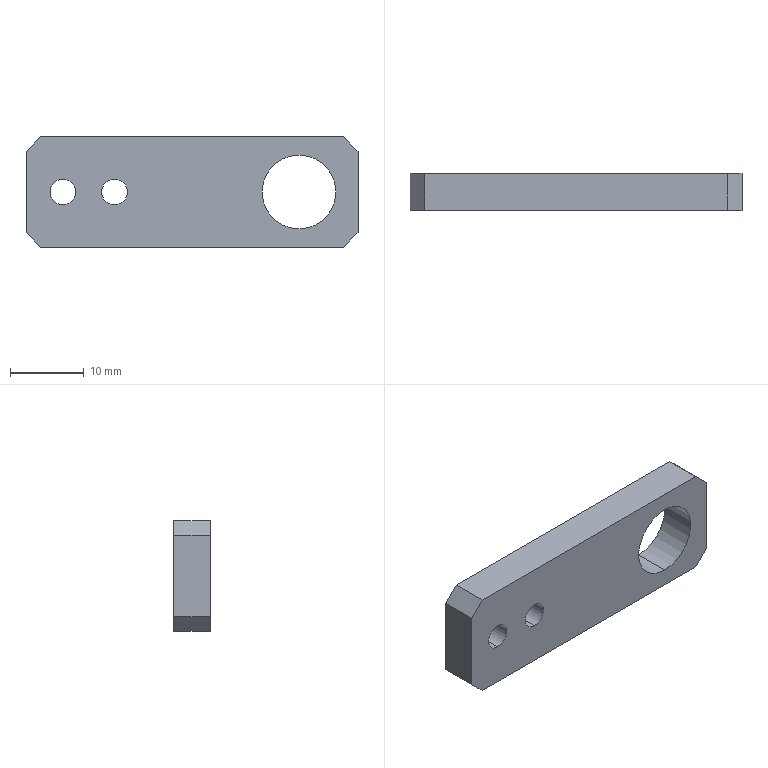Part | STEP file | Extension spring wire fixing bracket 1001 | 1 solid | 16 faces | box 45 x 5 x 15 mm | volume 2846 mm3 | plane 10 | cylinder 6 | commonest cylinder face diameters 3.5 x4 10 x2
STEP:
#1=CARTESIAN_POINT('',(0.,0.,0.));
#2=DIRECTION('',(0.,0.,1.));
#3=DIRECTION('',(1.,0.,0.));
#4=AXIS2_PLACEMENT_3D('',#1,#2,#3);
#5=CARTESIAN_POINT('',(-17.5,0.,1.75));
#6=VERTEX_POINT('',#5);
#7=CARTESIAN_POINT('',(-17.5,5.,1.75));
#8=VERTEX_POINT('',#7);
#9=CARTESIAN_POINT('',(-17.5,0.,1.75));
#10=DIRECTION('',(0.,1.,0.));
#11=VECTOR('',#10,1.);
#12=LINE('',#9,#11);
#13=CARTESIAN_POINT('',(-17.5,0.,0.));
#14=DIRECTION('',(0.,1.,0.));
#15=DIRECTION('',(0.,0.,1.));
#16=AXIS2_PLACEMENT_3D('',#13,#14,#15);
#17=CYLINDRICAL_SURFACE('',#16,1.75);
#18=CARTESIAN_POINT('',(6.283,0.));
#19=DIRECTION('',(0.,1.));
#20=VECTOR('',#19,1.);
#21=LINE('',#18,#20);
#22=(GEOMETRIC_REPRESENTATION_CONTEXT(2)PARAMETRIC_REPRESENTATION_CONTEXT()REPRESENTATION_CONTEXT('',''));
#23=DEFINITIONAL_REPRESENTATION('',(#21),#22);
#24=PCURVE('',#17,#23);
#25=CARTESIAN_POINT('',(-17.5,0.,0.));
#26=DIRECTION('',(0.,1.,0.));
#27=DIRECTION('',(0.,0.,1.));
#28=AXIS2_PLACEMENT_3D('',#25,#26,#27);
#29=CYLINDRICAL_SURFACE('',#28,1.75);
#30=CARTESIAN_POINT('',(0.,0.));
#31=DIRECTION('',(0.,1.));
#32=VECTOR('',#31,1.);
#33=LINE('',#30,#32);
#34=(GEOMETRIC_REPRESENTATION_CONTEXT(2)PARAMETRIC_REPRESENTATION_CONTEXT()REPRESENTATION_CONTEXT('',''));
#35=DEFINITIONAL_REPRESENTATION('',(#33),#34);
#36=PCURVE('',#29,#35);
#37=SURFACE_CURVE('',#12,(#24,#36),.PCURVE_S1.);
#38=EDGE_CURVE('',#6,#8,#37,.T.);
#39=ORIENTED_EDGE('',*,*,#38,.T.);
#40=CARTESIAN_POINT('',(-17.5,5.,-1.75));
#41=VERTEX_POINT('',#40);
#42=CARTESIAN_POINT('',(-17.5,5.,0.));
#43=DIRECTION('',(0.,1.,0.));
#44=DIRECTION('',(0.,0.,1.));
#45=AXIS2_PLACEMENT_3D('',#42,#43,#44);
#46=CIRCLE('',#45,1.75);
#47=CARTESIAN_POINT('',(0.,5.));
#48=DIRECTION('',(1.,0.));
#49=VECTOR('',#48,1.);
#50=LINE('',#47,#49);
#51=(GEOMETRIC_REPRESENTATION_CONTEXT(2)PARAMETRIC_REPRESENTATION_CONTEXT()REPRESENTATION_CONTEXT('',''));
#52=DEFINITIONAL_REPRESENTATION('',(#50),#51);
#53=PCURVE('',#17,#52);
#54=CARTESIAN_POINT('',(0.,5.,0.));
#55=DIRECTION('',(0.,-1.,0.));
#56=DIRECTION('',(0.,0.,-1.));
#57=AXIS2_PLACEMENT_3D('',#54,#55,#56);
#58=PLANE('',#57);
#59=CARTESIAN_POINT('',(-1.75,-17.5));
#60=CARTESIAN_POINT('',(-1.75,-14.469));
#61=CARTESIAN_POINT('',(0.875,-15.984));
#62=CARTESIAN_POINT('',(3.5,-17.5));
#63=CARTESIAN_POINT('',(0.875,-19.016));
#64=CARTESIAN_POINT('',(-1.75,-20.531));
#65=CARTESIAN_POINT('',(-1.75,-17.5));
#66=(BOUNDED_CURVE()B_SPLINE_CURVE(2,(#59,#60,#61,#62,#63,#64,#65),.UNSPECIFIED.,.T.,.F.)B_SPLINE_CURVE_WITH_KNOTS((1,2,2,2,2,1),(-2.094,0.,2.094,4.189,6.283,8.378),.UNSPECIFIED.)CURVE()GEOMETRIC_REPRESENTATION_ITEM()RATIONAL_B_SPLINE_CURVE((1.,0.5,1.,0.5,1.,0.5,1.))REPRESENTATION_ITEM(''));
#67=(GEOMETRIC_REPRESENTATION_CONTEXT(2)PARAMETRIC_REPRESENTATION_CONTEXT()REPRESENTATION_CONTEXT('',''));
#68=DEFINITIONAL_REPRESENTATION('',(#66),#67);
#69=PCURVE('',#58,#68);
#70=SURFACE_CURVE('',#46,(#53,#69),.PCURVE_S1.);
#71=EDGE_CURVE('',#41,#8,#70,.T.);
#72=ORIENTED_EDGE('',*,*,#71,.F.);
#73=CARTESIAN_POINT('',(-17.5,0.,-1.75));
#74=VERTEX_POINT('',#73);
#75=CARTESIAN_POINT('',(-17.5,0.,-1.75));
#76=DIRECTION('',(0.,1.,0.));
#77=VECTOR('',#76,1.);
#78=LINE('',#75,#77);
#79=CARTESIAN_POINT('',(3.142,0.));
#80=DIRECTION('',(0.,1.));
#81=VECTOR('',#80,1.);
#82=LINE('',#79,#81);
#83=(GEOMETRIC_REPRESENTATION_CONTEXT(2)PARAMETRIC_REPRESENTATION_CONTEXT()REPRESENTATION_CONTEXT('',''));
#84=DEFINITIONAL_REPRESENTATION('',(#82),#83);
#85=PCURVE('',#17,#84);
#86=CARTESIAN_POINT('',(3.142,0.));
#87=DIRECTION('',(0.,1.));
#88=VECTOR('',#87,1.);
#89=LINE('',#86,#88);
#90=(GEOMETRIC_REPRESENTATION_CONTEXT(2)PARAMETRIC_REPRESENTATION_CONTEXT()REPRESENTATION_CONTEXT('',''));
#91=DEFINITIONAL_REPRESENTATION('',(#89),#90);
#92=PCURVE('',#29,#91);
#93=SURFACE_CURVE('',#78,(#85,#92),.PCURVE_S1.);
#94=EDGE_CURVE('',#74,#41,#93,.T.);
#95=ORIENTED_EDGE('',*,*,#94,.F.);
#96=CARTESIAN_POINT('',(-17.5,0.,0.));
#97=DIRECTION('',(0.,1.,0.));
#98=DIRECTION('',(0.,0.,1.));
#99=AXIS2_PLACEMENT_3D('',#96,#97,#98);
#100=CIRCLE('',#99,1.75);
#101=CARTESIAN_POINT('',(0.,0.));
#102=DIRECTION('',(1.,0.));
#103=VECTOR('',#102,1.);
#104=LINE('',#101,#103);
#105=(GEOMETRIC_REPRESENTATION_CONTEXT(2)PARAMETRIC_REPRESENTATION_CONTEXT()REPRESENTATION_CONTEXT('',''));
#106=DEFINITIONAL_REPRESENTATION('',(#104),#105);
#107=PCURVE('',#17,#106);
#108=CARTESIAN_POINT('',(0.,0.,0.));
#109=DIRECTION('',(0.,-1.,0.));
#110=DIRECTION('',(0.,0.,-1.));
#111=AXIS2_PLACEMENT_3D('',#108,#109,#110);
#112=PLANE('',#111);
#113=CARTESIAN_POINT('',(-1.75,-17.5));
#114=CARTESIAN_POINT('',(-1.75,-14.469));
#115=CARTESIAN_POINT('',(0.875,-15.984));
#116=CARTESIAN_POINT('',(3.5,-17.5));
#117=CARTESIAN_POINT('',(0.875,-19.016));
#118=CARTESIAN_POINT('',(-1.75,-20.531));
#119=CARTESIAN_POINT('',(-1.75,-17.5));
#120=(BOUNDED_CURVE()B_SPLINE_CURVE(2,(#113,#114,#115,#116,#117,#118,#119),.UNSPECIFIED.,.T.,.F.)B_SPLINE_CURVE_WITH_KNOTS((1,2,2,2,2,1),(-2.094,0.,2.094,4.189,6.283,8.378),.UNSPECIFIED.)CURVE()GEOMETRIC_REPRESENTATION_ITEM()RATIONAL_B_SPLINE_CURVE((1.,0.5,1.,0.5,1.,0.5,1.))REPRESENTATION_ITEM(''));
#121=(GEOMETRIC_REPRESENTATION_CONTEXT(2)PARAMETRIC_REPRESENTATION_CONTEXT()REPRESENTATION_CONTEXT('',''));
#122=DEFINITIONAL_REPRESENTATION('',(#120),#121);
#123=PCURVE('',#112,#122);
#124=SURFACE_CURVE('',#100,(#107,#123),.PCURVE_S1.);
#125=EDGE_CURVE('',#74,#6,#124,.T.);
#126=ORIENTED_EDGE('',*,*,#125,.T.);
#127=EDGE_LOOP('',(#39,#72,#95,#126));
#128=FACE_BOUND('',#127,.F.);
#129=ADVANCED_FACE('',(#128),#17,.F.);
#130=CARTESIAN_POINT('',(-10.5,0.,1.75));
#131=VERTEX_POINT('',#130);
#132=CARTESIAN_POINT('',(-10.5,5.,1.75));
#133=VERTEX_POINT('',#132);
#134=CARTESIAN_POINT('',(-10.5,0.,1.75));
#135=DIRECTION('',(0.,1.,0.));
#136=VECTOR('',#135,1.);
#137=LINE('',#134,#136);
#138=CARTESIAN_POINT('',(-10.5,0.,0.));
#139=DIRECTION('',(0.,1.,0.));
#140=DIRECTION('',(0.,0.,1.));
#141=AXIS2_PLACEMENT_3D('',#138,#139,#140);
#142=CYLINDRICAL_SURFACE('',#141,1.75);
#143=CARTESIAN_POINT('',(6.283,0.));
#144=DIRECTION('',(0.,1.));
#145=VECTOR('',#144,1.);
#146=LINE('',#143,#145);
#147=(GEOMETRIC_REPRESENTATION_CONTEXT(2)PARAMETRIC_REPRESENTATION_CONTEXT()REPRESENTATION_CONTEXT('',''));
#148=DEFINITIONAL_REPRESENTATION('',(#146),#147);
#149=PCURVE('',#142,#148);
#150=CARTESIAN_POINT('',(-10.5,0.,0.));
#151=DIRECTION('',(0.,1.,0.));
#152=DIRECTION('',(0.,0.,1.));
#153=AXIS2_PLACEMENT_3D('',#150,#151,#152);
#154=CYLINDRICAL_SURFACE('',#153,1.75);
#155=CARTESIAN_POINT('',(0.,0.));
#156=DIRECTION('',(0.,1.));
#157=VECTOR('',#156,1.);
#158=LINE('',#155,#157);
#159=(GEOMETRIC_REPRESENTATION_CONTEXT(2)PARAMETRIC_REPRESENTATION_CONTEXT()REPRESENTATION_CONTEXT('',''));
#160=DEFINITIONAL_REPRESENTATION('',(#158),#159);
#161=PCURVE('',#154,#160);
#162=SURFACE_CURVE('',#137,(#149,#161),.PCURVE_S1.);
#163=EDGE_CURVE('',#131,#133,#162,.T.);
#164=ORIENTED_EDGE('',*,*,#163,.T.);
#165=CARTESIAN_POINT('',(-10.5,5.,-1.75));
#166=VERTEX_POINT('',#165);
#167=CARTESIAN_POINT('',(-10.5,5.,0.));
#168=DIRECTION('',(0.,1.,0.));
#169=DIRECTION('',(0.,0.,1.));
#170=AXIS2_PLACEMENT_3D('',#167,#168,#169);
#171=CIRCLE('',#170,1.75);
#172=CARTESIAN_POINT('',(0.,5.));
#173=DIRECTION('',(1.,0.));
#174=VECTOR('',#173,1.);
#175=LINE('',#172,#174);
#176=(GEOMETRIC_REPRESENTATION_CONTEXT(2)PARAMETRIC_REPRESENTATION_CONTEXT()REPRESENTATION_CONTEXT('',''));
#177=DEFINITIONAL_REPRESENTATION('',(#175),#176);
#178=PCURVE('',#142,#177);
#179=CARTESIAN_POINT('',(-1.75,-10.5));
#180=CARTESIAN_POINT('',(-1.75,-7.469));
#181=CARTESIAN_POINT('',(0.875,-8.984));
#182=CARTESIAN_POINT('',(3.5,-10.5));
#183=CARTESIAN_POINT('',(0.875,-12.016));
#184=CARTESIAN_POINT('',(-1.75,-13.531));
#185=CARTESIAN_POINT('',(-1.75,-10.5));
#186=(BOUNDED_CURVE()B_SPLINE_CURVE(2,(#179,#180,#181,#182,#183,#184,#185),.UNSPECIFIED.,.T.,.F.)B_SPLINE_CURVE_WITH_KNOTS((1,2,2,2,2,1),(-2.094,0.,2.094,4.189,6.283,8.378),.UNSPECIFIED.)CURVE()GEOMETRIC_REPRESENTATION_ITEM()RATIONAL_B_SPLINE_CURVE((1.,0.5,1.,0.5,1.,0.5,1.))REPRESENTATION_ITEM(''));
#187=(GEOMETRIC_REPRESENTATION_CONTEXT(2)PARAMETRIC_REPRESENTATION_CONTEXT()REPRESENTATION_CONTEXT('',''));
#188=DEFINITIONAL_REPRESENTATION('',(#186),#187);
#189=PCURVE('',#58,#188);
#190=SURFACE_CURVE('',#171,(#178,#189),.PCURVE_S1.);
#191=EDGE_CURVE('',#166,#133,#190,.T.);
#192=ORIENTED_EDGE('',*,*,#191,.F.);
#193=CARTESIAN_POINT('',(-10.5,0.,-1.75));
#194=VERTEX_POINT('',#193);
#195=CARTESIAN_POINT('',(-10.5,0.,-1.75));
#196=DIRECTION('',(0.,1.,0.));
#197=VECTOR('',#196,1.);
#198=LINE('',#195,#197);
#199=CARTESIAN_POINT('',(3.142,0.));
#200=DIRECTION('',(0.,1.));
#201=VECTOR('',#200,1.);
#202=LINE('',#199,#201);
#203=(GEOMETRIC_REPRESENTATION_CONTEXT(2)PARAMETRIC_REPRESENTATION_CONTEXT()REPRESENTATION_CONTEXT('',''));
#204=DEFINITIONAL_REPRESENTATION('',(#202),#203);
#205=PCURVE('',#142,#204);
#206=CARTESIAN_POINT('',(3.142,0.));
#207=DIRECTION('',(0.,1.));
#208=VECTOR('',#207,1.);
#209=LINE('',#206,#208);
#210=(GEOMETRIC_REPRESENTATION_CONTEXT(2)PARAMETRIC_REPRESENTATION_CONTEXT()REPRESENTATION_CONTEXT('',''));
#211=DEFINITIONAL_REPRESENTATION('',(#209),#210);
#212=PCURVE('',#154,#211);
#213=SURFACE_CURVE('',#198,(#205,#212),.PCURVE_S1.);
#214=EDGE_CURVE('',#194,#166,#213,.T.);
#215=ORIENTED_EDGE('',*,*,#214,.F.);
#216=CARTESIAN_POINT('',(-10.5,0.,0.));
#217=DIRECTION('',(0.,1.,0.));
#218=DIRECTION('',(0.,0.,1.));
#219=AXIS2_PLACEMENT_3D('',#216,#217,#218);
#220=CIRCLE('',#219,1.75);
#221=CARTESIAN_POINT('',(0.,0.));
#222=DIRECTION('',(1.,0.));
#223=VECTOR('',#222,1.);
#224=LINE('',#221,#223);
#225=(GEOMETRIC_REPRESENTATION_CONTEXT(2)PARAMETRIC_REPRESENTATION_CONTEXT()REPRESENTATION_CONTEXT('',''));
#226=DEFINITIONAL_REPRESENTATION('',(#224),#225);
#227=PCURVE('',#142,#226);
#228=CARTESIAN_POINT('',(-1.75,-10.5));
#229=CARTESIAN_POINT('',(-1.75,-7.469));
#230=CARTESIAN_POINT('',(0.875,-8.984));
#231=CARTESIAN_POINT('',(3.5,-10.5));
#232=CARTESIAN_POINT('',(0.875,-12.016));
#233=CARTESIAN_POINT('',(-1.75,-13.531));
#234=CARTESIAN_POINT('',(-1.75,-10.5));
#235=(BOUNDED_CURVE()B_SPLINE_CURVE(2,(#228,#229,#230,#231,#232,#233,#234),.UNSPECIFIED.,.T.,.F.)B_SPLINE_CURVE_WITH_KNOTS((1,2,2,2,2,1),(-2.094,0.,2.094,4.189,6.283,8.378),.UNSPECIFIED.)CURVE()GEOMETRIC_REPRESENTATION_ITEM()RATIONAL_B_SPLINE_CURVE((1.,0.5,1.,0.5,1.,0.5,1.))REPRESENTATION_ITEM(''));
#236=(GEOMETRIC_REPRESENTATION_CONTEXT(2)PARAMETRIC_REPRESENTATION_CONTEXT()REPRESENTATION_CONTEXT('',''));
#237=DEFINITIONAL_REPRESENTATION('',(#235),#236);
#238=PCURVE('',#112,#237);
#239=SURFACE_CURVE('',#220,(#227,#238),.PCURVE_S1.);
#240=EDGE_CURVE('',#194,#131,#239,.T.);
#241=ORIENTED_EDGE('',*,*,#240,.T.);
#242=EDGE_LOOP('',(#164,#192,#215,#241));
#243=FACE_BOUND('',#242,.F.);
#244=ADVANCED_FACE('',(#243),#142,.F.);
#245=CARTESIAN_POINT('',(14.5,0.,5.));
#246=VERTEX_POINT('',#245);
#247=CARTESIAN_POINT('',(14.5,5.,5.));
#248=VERTEX_POINT('',#247);
#249=CARTESIAN_POINT('',(14.5,0.,5.));
#250=DIRECTION('',(0.,1.,0.));
#251=VECTOR('',#250,1.);
#252=LINE('',#249,#251);
#253=CARTESIAN_POINT('',(14.5,0.,0.));
#254=DIRECTION('',(0.,1.,0.));
#255=DIRECTION('',(0.,0.,1.));
#256=AXIS2_PLACEMENT_3D('',#253,#254,#255);
#257=CYLINDRICAL_SURFACE('',#256,5.);
#258=CARTESIAN_POINT('',(6.283,0.));
#259=DIRECTION('',(0.,1.));
#260=VECTOR('',#259,1.);
#261=LINE('',#258,#260);
#262=(GEOMETRIC_REPRESENTATION_CONTEXT(2)PARAMETRIC_REPRESENTATION_CONTEXT()REPRESENTATION_CONTEXT('',''));
#263=DEFINITIONAL_REPRESENTATION('',(#261),#262);
#264=PCURVE('',#257,#263);
#265=CARTESIAN_POINT('',(14.5,0.,0.));
#266=DIRECTION('',(0.,1.,0.));
#267=DIRECTION('',(0.,0.,1.));
#268=AXIS2_PLACEMENT_3D('',#265,#266,#267);
#269=CYLINDRICAL_SURFACE('',#268,5.);
#270=CARTESIAN_POINT('',(0.,0.));
#271=DIRECTION('',(0.,1.));
#272=VECTOR('',#271,1.);
#273=LINE('',#270,#272);
#274=(GEOMETRIC_REPRESENTATION_CONTEXT(2)PARAMETRIC_REPRESENTATION_CONTEXT()REPRESENTATION_CONTEXT('',''));
#275=DEFINITIONAL_REPRESENTATION('',(#273),#274);
#276=PCURVE('',#269,#275);
#277=SURFACE_CURVE('',#252,(#264,#276),.PCURVE_S1.);
#278=EDGE_CURVE('',#246,#248,#277,.T.);
#279=ORIENTED_EDGE('',*,*,#278,.T.);
#280=CARTESIAN_POINT('',(14.5,5.,-5.));
#281=VERTEX_POINT('',#280);
#282=CARTESIAN_POINT('',(14.5,5.,0.));
#283=DIRECTION('',(0.,1.,0.));
#284=DIRECTION('',(0.,0.,1.));
#285=AXIS2_PLACEMENT_3D('',#282,#283,#284);
#286=CIRCLE('',#285,5.);
#287=CARTESIAN_POINT('',(0.,5.));
#288=DIRECTION('',(1.,0.));
#289=VECTOR('',#288,1.);
#290=LINE('',#287,#289);
#291=(GEOMETRIC_REPRESENTATION_CONTEXT(2)PARAMETRIC_REPRESENTATION_CONTEXT()REPRESENTATION_CONTEXT('',''));
#292=DEFINITIONAL_REPRESENTATION('',(#290),#291);
#293=PCURVE('',#257,#292);
#294=CARTESIAN_POINT('',(-5.,14.5));
#295=CARTESIAN_POINT('',(-5.,23.16));
#296=CARTESIAN_POINT('',(2.5,18.83));
#297=CARTESIAN_POINT('',(10.,14.5));
#298=CARTESIAN_POINT('',(2.5,10.17));
#299=CARTESIAN_POINT('',(-5.,5.84));
#300=CARTESIAN_POINT('',(-5.,14.5));
#301=(BOUNDED_CURVE()B_SPLINE_CURVE(2,(#294,#295,#296,#297,#298,#299,#300),.UNSPECIFIED.,.T.,.F.)B_SPLINE_CURVE_WITH_KNOTS((1,2,2,2,2,1),(-2.094,0.,2.094,4.189,6.283,8.378),.UNSPECIFIED.)CURVE()GEOMETRIC_REPRESENTATION_ITEM()RATIONAL_B_SPLINE_CURVE((1.,0.5,1.,0.5,1.,0.5,1.))REPRESENTATION_ITEM(''));
#302=(GEOMETRIC_REPRESENTATION_CONTEXT(2)PARAMETRIC_REPRESENTATION_CONTEXT()REPRESENTATION_CONTEXT('',''));
#303=DEFINITIONAL_REPRESENTATION('',(#301),#302);
#304=PCURVE('',#58,#303);
#305=SURFACE_CURVE('',#286,(#293,#304),.PCURVE_S1.);
#306=EDGE_CURVE('',#281,#248,#305,.T.);
#307=ORIENTED_EDGE('',*,*,#306,.F.);
#308=CARTESIAN_POINT('',(14.5,0.,-5.));
#309=VERTEX_POINT('',#308);
#310=CARTESIAN_POINT('',(14.5,0.,-5.));
#311=DIRECTION('',(0.,1.,0.));
#312=VECTOR('',#311,1.);
#313=LINE('',#310,#312);
#314=CARTESIAN_POINT('',(3.142,0.));
#315=DIRECTION('',(0.,1.));
#316=VECTOR('',#315,1.);
#317=LINE('',#314,#316);
#318=(GEOMETRIC_REPRESENTATION_CONTEXT(2)PARAMETRIC_REPRESENTATION_CONTEXT()REPRESENTATION_CONTEXT('',''));
#319=DEFINITIONAL_REPRESENTATION('',(#317),#318);
#320=PCURVE('',#257,#319);
#321=CARTESIAN_POINT('',(3.142,0.));
#322=DIRECTION('',(0.,1.));
#323=VECTOR('',#322,1.);
#324=LINE('',#321,#323);
#325=(GEOMETRIC_REPRESENTATION_CONTEXT(2)PARAMETRIC_REPRESENTATION_CONTEXT()REPRESENTATION_CONTEXT('',''));
#326=DEFINITIONAL_REPRESENTATION('',(#324),#325);
#327=PCURVE('',#269,#326);
#328=SURFACE_CURVE('',#313,(#320,#327),.PCURVE_S1.);
#329=EDGE_CURVE('',#309,#281,#328,.T.);
#330=ORIENTED_EDGE('',*,*,#329,.F.);
#331=CARTESIAN_POINT('',(14.5,0.,0.));
#332=DIRECTION('',(0.,1.,0.));
#333=DIRECTION('',(0.,0.,1.));
#334=AXIS2_PLACEMENT_3D('',#331,#332,#333);
#335=CIRCLE('',#334,5.);
#336=CARTESIAN_POINT('',(0.,0.));
#337=DIRECTION('',(1.,0.));
#338=VECTOR('',#337,1.);
#339=LINE('',#336,#338);
#340=(GEOMETRIC_REPRESENTATION_CONTEXT(2)PARAMETRIC_REPRESENTATION_CONTEXT()REPRESENTATION_CONTEXT('',''));
#341=DEFINITIONAL_REPRESENTATION('',(#339),#340);
#342=PCURVE('',#257,#341);
#343=CARTESIAN_POINT('',(-5.,14.5));
#344=CARTESIAN_POINT('',(-5.,23.16));
#345=CARTESIAN_POINT('',(2.5,18.83));
#346=CARTESIAN_POINT('',(10.,14.5));
#347=CARTESIAN_POINT('',(2.5,10.17));
#348=CARTESIAN_POINT('',(-5.,5.84));
#349=CARTESIAN_POINT('',(-5.,14.5));
#350=(BOUNDED_CURVE()B_SPLINE_CURVE(2,(#343,#344,#345,#346,#347,#348,#349),.UNSPECIFIED.,.T.,.F.)B_SPLINE_CURVE_WITH_KNOTS((1,2,2,2,2,1),(-2.094,0.,2.094,4.189,6.283,8.378),.UNSPECIFIED.)CURVE()GEOMETRIC_REPRESENTATION_ITEM()RATIONAL_B_SPLINE_CURVE((1.,0.5,1.,0.5,1.,0.5,1.))REPRESENTATION_ITEM(''));
#351=(GEOMETRIC_REPRESENTATION_CONTEXT(2)PARAMETRIC_REPRESENTATION_CONTEXT()REPRESENTATION_CONTEXT('',''));
#352=DEFINITIONAL_REPRESENTATION('',(#350),#351);
#353=PCURVE('',#112,#352);
#354=SURFACE_CURVE('',#335,(#342,#353),.PCURVE_S1.);
#355=EDGE_CURVE('',#309,#246,#354,.T.);
#356=ORIENTED_EDGE('',*,*,#355,.T.);
#357=EDGE_LOOP('',(#279,#307,#330,#356));
#358=FACE_BOUND('',#357,.F.);
#359=ADVANCED_FACE('',(#358),#257,.F.);
#360=CARTESIAN_POINT('',(22.5,5.,5.5));
#361=VERTEX_POINT('',#360);
#362=CARTESIAN_POINT('',(22.5,5.,-5.5));
#363=VERTEX_POINT('',#362);
#364=CARTESIAN_POINT('',(22.5,5.,7.5));
#365=DIRECTION('',(0.,0.,-1.));
#366=VECTOR('',#365,1.);
#367=LINE('',#364,#366);
#368=CARTESIAN_POINT('',(22.5,5.,7.5));
#369=DIRECTION('',(-1.,0.,0.));
#370=DIRECTION('',(0.,0.,1.));
#371=AXIS2_PLACEMENT_3D('',#368,#369,#370);
#372=PLANE('',#371);
#373=CARTESIAN_POINT('',(0.,0.));
#374=DIRECTION('',(-1.,0.));
#375=VECTOR('',#374,1.);
#376=LINE('',#373,#375);
#377=(GEOMETRIC_REPRESENTATION_CONTEXT(2)PARAMETRIC_REPRESENTATION_CONTEXT()REPRESENTATION_CONTEXT('',''));
#378=DEFINITIONAL_REPRESENTATION('',(#376),#377);
#379=PCURVE('',#372,#378);
#380=CARTESIAN_POINT('',(-7.5,22.5));
#381=DIRECTION('',(1.,0.));
#382=VECTOR('',#381,1.);
#383=LINE('',#380,#382);
#384=(GEOMETRIC_REPRESENTATION_CONTEXT(2)PARAMETRIC_REPRESENTATION_CONTEXT()REPRESENTATION_CONTEXT('',''));
#385=DEFINITIONAL_REPRESENTATION('',(#383),#384);
#386=PCURVE('',#58,#385);
#387=SURFACE_CURVE('',#367,(#379,#386),.PCURVE_S1.);
#388=EDGE_CURVE('',#361,#363,#387,.T.);
#389=ORIENTED_EDGE('',*,*,#388,.F.);
#390=CARTESIAN_POINT('',(22.5,0.,5.5));
#391=VERTEX_POINT('',#390);
#392=CARTESIAN_POINT('',(22.5,5.,5.5));
#393=DIRECTION('',(0.,-1.,0.));
#394=VECTOR('',#393,1.);
#395=LINE('',#392,#394);
#396=CARTESIAN_POINT('',(-2.,0.));
#397=DIRECTION('',(0.,-1.));
#398=VECTOR('',#397,1.);
#399=LINE('',#396,#398);
#400=(GEOMETRIC_REPRESENTATION_CONTEXT(2)PARAMETRIC_REPRESENTATION_CONTEXT()REPRESENTATION_CONTEXT('',''));
#401=DEFINITIONAL_REPRESENTATION('',(#399),#400);
#402=PCURVE('',#372,#401);
#403=CARTESIAN_POINT('',(22.5,5.,5.5));
#404=DIRECTION('',(-0.7071,0.,-0.7071));
#405=DIRECTION('',(0.,-1.,0.));
#406=AXIS2_PLACEMENT_3D('',#403,#404,#405);
#407=PLANE('',#406);
#408=CARTESIAN_POINT('',(0.,0.));
#409=DIRECTION('',(1.,0.));
#410=VECTOR('',#409,1.);
#411=LINE('',#408,#410);
#412=(GEOMETRIC_REPRESENTATION_CONTEXT(2)PARAMETRIC_REPRESENTATION_CONTEXT()REPRESENTATION_CONTEXT('',''));
#413=DEFINITIONAL_REPRESENTATION('',(#411),#412);
#414=PCURVE('',#407,#413);
#415=SURFACE_CURVE('',#395,(#402,#414),.PCURVE_S1.);
#416=EDGE_CURVE('',#361,#391,#415,.T.);
#417=ORIENTED_EDGE('',*,*,#416,.T.);
#418=CARTESIAN_POINT('',(22.5,0.,-5.5));
#419=VERTEX_POINT('',#418);
#420=CARTESIAN_POINT('',(22.5,0.,7.5));
#421=DIRECTION('',(0.,0.,-1.));
#422=VECTOR('',#421,1.);
#423=LINE('',#420,#422);
#424=CARTESIAN_POINT('',(0.,-5.));
#425=DIRECTION('',(-1.,0.));
#426=VECTOR('',#425,1.);
#427=LINE('',#424,#426);
#428=(GEOMETRIC_REPRESENTATION_CONTEXT(2)PARAMETRIC_REPRESENTATION_CONTEXT()REPRESENTATION_CONTEXT('',''));
#429=DEFINITIONAL_REPRESENTATION('',(#427),#428);
#430=PCURVE('',#372,#429);
#431=CARTESIAN_POINT('',(-7.5,22.5));
#432=DIRECTION('',(1.,0.));
#433=VECTOR('',#432,1.);
#434=LINE('',#431,#433);
#435=(GEOMETRIC_REPRESENTATION_CONTEXT(2)PARAMETRIC_REPRESENTATION_CONTEXT()REPRESENTATION_CONTEXT('',''));
#436=DEFINITIONAL_REPRESENTATION('',(#434),#435);
#437=PCURVE('',#112,#436);
#438=SURFACE_CURVE('',#423,(#430,#437),.PCURVE_S1.);
#439=EDGE_CURVE('',#391,#419,#438,.T.);
#440=ORIENTED_EDGE('',*,*,#439,.T.);
#441=CARTESIAN_POINT('',(22.5,5.,-5.5));
#442=DIRECTION('',(0.,1.,0.));
#443=VECTOR('',#442,1.);
#444=LINE('',#441,#443);
#445=CARTESIAN_POINT('',(-13.,0.));
#446=DIRECTION('',(0.,1.));
#447=VECTOR('',#446,1.);
#448=LINE('',#445,#447);
#449=(GEOMETRIC_REPRESENTATION_CONTEXT(2)PARAMETRIC_REPRESENTATION_CONTEXT()REPRESENTATION_CONTEXT('',''));
#450=DEFINITIONAL_REPRESENTATION('',(#448),#449);
#451=PCURVE('',#372,#450);
#452=CARTESIAN_POINT('',(20.5,5.,-7.5));
#453=DIRECTION('',(-0.7071,0.,0.7071));
#454=DIRECTION('',(0.,-1.,0.));
#455=AXIS2_PLACEMENT_3D('',#452,#453,#454);
#456=PLANE('',#455);
#457=CARTESIAN_POINT('',(0.,2.828));
#458=DIRECTION('',(-1.,0.));
#459=VECTOR('',#458,1.);
#460=LINE('',#457,#459);
#461=(GEOMETRIC_REPRESENTATION_CONTEXT(2)PARAMETRIC_REPRESENTATION_CONTEXT()REPRESENTATION_CONTEXT('',''));
#462=DEFINITIONAL_REPRESENTATION('',(#460),#461);
#463=PCURVE('',#456,#462);
#464=SURFACE_CURVE('',#444,(#451,#463),.PCURVE_S1.);
#465=EDGE_CURVE('',#419,#363,#464,.T.);
#466=ORIENTED_EDGE('',*,*,#465,.T.);
#467=EDGE_LOOP('',(#389,#417,#440,#466));
#468=FACE_BOUND('',#467,.T.);
#469=ADVANCED_FACE('',(#468),#372,.F.);
#470=CARTESIAN_POINT('',(20.5,0.,-7.5));
#471=VERTEX_POINT('',#470);
#472=CARTESIAN_POINT('',(-20.5,0.,-7.5));
#473=VERTEX_POINT('',#472);
#474=CARTESIAN_POINT('',(-22.5,0.,-7.5));
#475=DIRECTION('',(-1.,0.,0.));
#476=VECTOR('',#475,1.);
#477=LINE('',#474,#476);
#478=CARTESIAN_POINT('',(-22.5,5.,-7.5));
#479=DIRECTION('',(0.,0.,1.));
#480=DIRECTION('',(1.,0.,0.));
#481=AXIS2_PLACEMENT_3D('',#478,#479,#480);
#482=PLANE('',#481);
#483=CARTESIAN_POINT('',(0.,-5.));
#484=DIRECTION('',(-1.,0.));
#485=VECTOR('',#484,1.);
#486=LINE('',#483,#485);
#487=(GEOMETRIC_REPRESENTATION_CONTEXT(2)PARAMETRIC_REPRESENTATION_CONTEXT()REPRESENTATION_CONTEXT('',''));
#488=DEFINITIONAL_REPRESENTATION('',(#486),#487);
#489=PCURVE('',#482,#488);
#490=CARTESIAN_POINT('',(7.5,-22.5));
#491=DIRECTION('',(0.,-1.));
#492=VECTOR('',#491,1.);
#493=LINE('',#490,#492);
#494=(GEOMETRIC_REPRESENTATION_CONTEXT(2)PARAMETRIC_REPRESENTATION_CONTEXT()REPRESENTATION_CONTEXT('',''));
#495=DEFINITIONAL_REPRESENTATION('',(#493),#494);
#496=PCURVE('',#112,#495);
#497=SURFACE_CURVE('',#477,(#489,#496),.PCURVE_S1.);
#498=EDGE_CURVE('',#471,#473,#497,.T.);
#499=ORIENTED_EDGE('',*,*,#498,.T.);
#500=CARTESIAN_POINT('',(-20.5,5.,-7.5));
#501=VERTEX_POINT('',#500);
#502=CARTESIAN_POINT('',(-20.5,5.,-7.5));
#503=DIRECTION('',(0.,1.,0.));
#504=VECTOR('',#503,1.);
#505=LINE('',#502,#504);
#506=CARTESIAN_POINT('',(2.,0.));
#507=DIRECTION('',(0.,1.));
#508=VECTOR('',#507,1.);
#509=LINE('',#506,#508);
#510=(GEOMETRIC_REPRESENTATION_CONTEXT(2)PARAMETRIC_REPRESENTATION_CONTEXT()REPRESENTATION_CONTEXT('',''));
#511=DEFINITIONAL_REPRESENTATION('',(#509),#510);
#512=PCURVE('',#482,#511);
#513=CARTESIAN_POINT('',(-22.5,5.,-5.5));
#514=DIRECTION('',(0.7071,0.,0.7071));
#515=DIRECTION('',(0.,-1.,0.));
#516=AXIS2_PLACEMENT_3D('',#513,#514,#515);
#517=PLANE('',#516);
#518=CARTESIAN_POINT('',(0.,2.828));
#519=DIRECTION('',(-1.,0.));
#520=VECTOR('',#519,1.);
#521=LINE('',#518,#520);
#522=(GEOMETRIC_REPRESENTATION_CONTEXT(2)PARAMETRIC_REPRESENTATION_CONTEXT()REPRESENTATION_CONTEXT('',''));
#523=DEFINITIONAL_REPRESENTATION('',(#521),#522);
#524=PCURVE('',#517,#523);
#525=SURFACE_CURVE('',#505,(#512,#524),.PCURVE_S1.);
#526=EDGE_CURVE('',#473,#501,#525,.T.);
#527=ORIENTED_EDGE('',*,*,#526,.T.);
#528=CARTESIAN_POINT('',(20.5,5.,-7.5));
#529=VERTEX_POINT('',#528);
#530=CARTESIAN_POINT('',(-22.5,5.,-7.5));
#531=DIRECTION('',(-1.,0.,0.));
#532=VECTOR('',#531,1.);
#533=LINE('',#530,#532);
#534=CARTESIAN_POINT('',(0.,0.));
#535=DIRECTION('',(-1.,0.));
#536=VECTOR('',#535,1.);
#537=LINE('',#534,#536);
#538=(GEOMETRIC_REPRESENTATION_CONTEXT(2)PARAMETRIC_REPRESENTATION_CONTEXT()REPRESENTATION_CONTEXT('',''));
#539=DEFINITIONAL_REPRESENTATION('',(#537),#538);
#540=PCURVE('',#482,#539);
#541=CARTESIAN_POINT('',(7.5,-22.5));
#542=DIRECTION('',(0.,-1.));
#543=VECTOR('',#542,1.);
#544=LINE('',#541,#543);
#545=(GEOMETRIC_REPRESENTATION_CONTEXT(2)PARAMETRIC_REPRESENTATION_CONTEXT()REPRESENTATION_CONTEXT('',''));
#546=DEFINITIONAL_REPRESENTATION('',(#544),#545);
#547=PCURVE('',#58,#546);
#548=SURFACE_CURVE('',#533,(#540,#547),.PCURVE_S1.);
#549=EDGE_CURVE('',#529,#501,#548,.T.);
#550=ORIENTED_EDGE('',*,*,#549,.F.);
#551=CARTESIAN_POINT('',(20.5,5.,-7.5));
#552=DIRECTION('',(0.,-1.,0.));
#553=VECTOR('',#552,1.);
#554=LINE('',#551,#553);
#555=CARTESIAN_POINT('',(43.,0.));
#556=DIRECTION('',(0.,-1.));
#557=VECTOR('',#556,1.);
#558=LINE('',#555,#557);
#559=(GEOMETRIC_REPRESENTATION_CONTEXT(2)PARAMETRIC_REPRESENTATION_CONTEXT()REPRESENTATION_CONTEXT('',''));
#560=DEFINITIONAL_REPRESENTATION('',(#558),#559);
#561=PCURVE('',#482,#560);
#562=CARTESIAN_POINT('',(0.,0.));
#563=DIRECTION('',(1.,0.));
#564=VECTOR('',#563,1.);
#565=LINE('',#562,#564);
#566=(GEOMETRIC_REPRESENTATION_CONTEXT(2)PARAMETRIC_REPRESENTATION_CONTEXT()REPRESENTATION_CONTEXT('',''));
#567=DEFINITIONAL_REPRESENTATION('',(#565),#566);
#568=PCURVE('',#456,#567);
#569=SURFACE_CURVE('',#554,(#561,#568),.PCURVE_S1.);
#570=EDGE_CURVE('',#529,#471,#569,.T.);
#571=ORIENTED_EDGE('',*,*,#570,.T.);
#572=EDGE_LOOP('',(#499,#527,#550,#571));
#573=FACE_BOUND('',#572,.T.);
#574=ADVANCED_FACE('',(#573),#482,.F.);
#575=CARTESIAN_POINT('',(-22.5,0.,-5.5));
#576=VERTEX_POINT('',#575);
#577=CARTESIAN_POINT('',(-22.5,0.,5.5));
#578=VERTEX_POINT('',#577);
#579=CARTESIAN_POINT('',(-22.5,0.,7.5));
#580=DIRECTION('',(0.,0.,1.));
#581=VECTOR('',#580,1.);
#582=LINE('',#579,#581);
#583=CARTESIAN_POINT('',(-22.5,5.,7.5));
#584=DIRECTION('',(1.,0.,0.));
#585=DIRECTION('',(0.,0.,-1.));
#586=AXIS2_PLACEMENT_3D('',#583,#584,#585);
#587=PLANE('',#586);
#588=CARTESIAN_POINT('',(0.,-5.));
#589=DIRECTION('',(-1.,0.));
#590=VECTOR('',#589,1.);
#591=LINE('',#588,#590);
#592=(GEOMETRIC_REPRESENTATION_CONTEXT(2)PARAMETRIC_REPRESENTATION_CONTEXT()REPRESENTATION_CONTEXT('',''));
#593=DEFINITIONAL_REPRESENTATION('',(#591),#592);
#594=PCURVE('',#587,#593);
#595=CARTESIAN_POINT('',(-7.5,-22.5));
#596=DIRECTION('',(-1.,0.));
#597=VECTOR('',#596,1.);
#598=LINE('',#595,#597);
#599=(GEOMETRIC_REPRESENTATION_CONTEXT(2)PARAMETRIC_REPRESENTATION_CONTEXT()REPRESENTATION_CONTEXT('',''));
#600=DEFINITIONAL_REPRESENTATION('',(#598),#599);
#601=PCURVE('',#112,#600);
#602=SURFACE_CURVE('',#582,(#594,#601),.PCURVE_S1.);
#603=EDGE_CURVE('',#576,#578,#602,.T.);
#604=ORIENTED_EDGE('',*,*,#603,.T.);
#605=CARTESIAN_POINT('',(-22.5,5.,5.5));
#606=VERTEX_POINT('',#605);
#607=CARTESIAN_POINT('',(-22.5,5.,5.5));
#608=DIRECTION('',(0.,1.,0.));
#609=VECTOR('',#608,1.);
#610=LINE('',#607,#609);
#611=CARTESIAN_POINT('',(2.,0.));
#612=DIRECTION('',(0.,1.));
#613=VECTOR('',#612,1.);
#614=LINE('',#611,#613);
#615=(GEOMETRIC_REPRESENTATION_CONTEXT(2)PARAMETRIC_REPRESENTATION_CONTEXT()REPRESENTATION_CONTEXT('',''));
#616=DEFINITIONAL_REPRESENTATION('',(#614),#615);
#617=PCURVE('',#587,#616);
#618=CARTESIAN_POINT('',(-20.5,5.,7.5));
#619=DIRECTION('',(0.7071,0.,-0.7071));
#620=DIRECTION('',(0.,-1.,0.));
#621=AXIS2_PLACEMENT_3D('',#618,#619,#620);
#622=PLANE('',#621);
#623=CARTESIAN_POINT('',(0.,2.828));
#624=DIRECTION('',(-1.,0.));
#625=VECTOR('',#624,1.);
#626=LINE('',#623,#625);
#627=(GEOMETRIC_REPRESENTATION_CONTEXT(2)PARAMETRIC_REPRESENTATION_CONTEXT()REPRESENTATION_CONTEXT('',''));
#628=DEFINITIONAL_REPRESENTATION('',(#626),#627);
#629=PCURVE('',#622,#628);
#630=SURFACE_CURVE('',#610,(#617,#629),.PCURVE_S1.);
#631=EDGE_CURVE('',#578,#606,#630,.T.);
#632=ORIENTED_EDGE('',*,*,#631,.T.);
#633=CARTESIAN_POINT('',(-22.5,5.,-5.5));
#634=VERTEX_POINT('',#633);
#635=CARTESIAN_POINT('',(-22.5,5.,7.5));
#636=DIRECTION('',(0.,0.,1.));
#637=VECTOR('',#636,1.);
#638=LINE('',#635,#637);
#639=CARTESIAN_POINT('',(0.,0.));
#640=DIRECTION('',(-1.,0.));
#641=VECTOR('',#640,1.);
#642=LINE('',#639,#641);
#643=(GEOMETRIC_REPRESENTATION_CONTEXT(2)PARAMETRIC_REPRESENTATION_CONTEXT()REPRESENTATION_CONTEXT('',''));
#644=DEFINITIONAL_REPRESENTATION('',(#642),#643);
#645=PCURVE('',#587,#644);
#646=CARTESIAN_POINT('',(-7.5,-22.5));
#647=DIRECTION('',(-1.,0.));
#648=VECTOR('',#647,1.);
#649=LINE('',#646,#648);
#650=(GEOMETRIC_REPRESENTATION_CONTEXT(2)PARAMETRIC_REPRESENTATION_CONTEXT()REPRESENTATION_CONTEXT('',''));
#651=DEFINITIONAL_REPRESENTATION('',(#649),#650);
#652=PCURVE('',#58,#651);
#653=SURFACE_CURVE('',#638,(#645,#652),.PCURVE_S1.);
#654=EDGE_CURVE('',#634,#606,#653,.T.);
#655=ORIENTED_EDGE('',*,*,#654,.F.);
#656=CARTESIAN_POINT('',(-22.5,5.,-5.5));
#657=DIRECTION('',(0.,-1.,0.));
#658=VECTOR('',#657,1.);
#659=LINE('',#656,#658);
#660=CARTESIAN_POINT('',(13.,0.));
#661=DIRECTION('',(0.,-1.));
#662=VECTOR('',#661,1.);
#663=LINE('',#660,#662);
#664=(GEOMETRIC_REPRESENTATION_CONTEXT(2)PARAMETRIC_REPRESENTATION_CONTEXT()REPRESENTATION_CONTEXT('',''));
#665=DEFINITIONAL_REPRESENTATION('',(#663),#664);
#666=PCURVE('',#587,#665);
#667=CARTESIAN_POINT('',(0.,0.));
#668=DIRECTION('',(1.,0.));
#669=VECTOR('',#668,1.);
#670=LINE('',#667,#669);
#671=(GEOMETRIC_REPRESENTATION_CONTEXT(2)PARAMETRIC_REPRESENTATION_CONTEXT()REPRESENTATION_CONTEXT('',''));
#672=DEFINITIONAL_REPRESENTATION('',(#670),#671);
#673=PCURVE('',#517,#672);
#674=SURFACE_CURVE('',#659,(#666,#673),.PCURVE_S1.);
#675=EDGE_CURVE('',#634,#576,#674,.T.);
#676=ORIENTED_EDGE('',*,*,#675,.T.);
#677=EDGE_LOOP('',(#604,#632,#655,#676));
#678=FACE_BOUND('',#677,.T.);
#679=ADVANCED_FACE('',(#678),#587,.F.);
#680=CARTESIAN_POINT('',(-20.5,0.,7.5));
#681=VERTEX_POINT('',#680);
#682=CARTESIAN_POINT('',(20.5,0.,7.5));
#683=VERTEX_POINT('',#682);
#684=CARTESIAN_POINT('',(-22.5,0.,7.5));
#685=DIRECTION('',(1.,0.,0.));
#686=VECTOR('',#685,1.);
#687=LINE('',#684,#686);
#688=CARTESIAN_POINT('',(-22.5,5.,7.5));
#689=DIRECTION('',(0.,0.,-1.));
#690=DIRECTION('',(-1.,0.,0.));
#691=AXIS2_PLACEMENT_3D('',#688,#689,#690);
#692=PLANE('',#691);
#693=CARTESIAN_POINT('',(0.,-5.));
#694=DIRECTION('',(-1.,0.));
#695=VECTOR('',#694,1.);
#696=LINE('',#693,#695);
#697=(GEOMETRIC_REPRESENTATION_CONTEXT(2)PARAMETRIC_REPRESENTATION_CONTEXT()REPRESENTATION_CONTEXT('',''));
#698=DEFINITIONAL_REPRESENTATION('',(#696),#697);
#699=PCURVE('',#692,#698);
#700=CARTESIAN_POINT('',(-7.5,-22.5));
#701=DIRECTION('',(0.,1.));
#702=VECTOR('',#701,1.);
#703=LINE('',#700,#702);
#704=(GEOMETRIC_REPRESENTATION_CONTEXT(2)PARAMETRIC_REPRESENTATION_CONTEXT()REPRESENTATION_CONTEXT('',''));
#705=DEFINITIONAL_REPRESENTATION('',(#703),#704);
#706=PCURVE('',#112,#705);
#707=SURFACE_CURVE('',#687,(#699,#706),.PCURVE_S1.);
#708=EDGE_CURVE('',#681,#683,#707,.T.);
#709=ORIENTED_EDGE('',*,*,#708,.T.);
#710=CARTESIAN_POINT('',(20.5,5.,7.5));
#711=VERTEX_POINT('',#710);
#712=CARTESIAN_POINT('',(20.5,5.,7.5));
#713=DIRECTION('',(0.,1.,0.));
#714=VECTOR('',#713,1.);
#715=LINE('',#712,#714);
#716=CARTESIAN_POINT('',(-43.,0.));
#717=DIRECTION('',(0.,1.));
#718=VECTOR('',#717,1.);
#719=LINE('',#716,#718);
#720=(GEOMETRIC_REPRESENTATION_CONTEXT(2)PARAMETRIC_REPRESENTATION_CONTEXT()REPRESENTATION_CONTEXT('',''));
#721=DEFINITIONAL_REPRESENTATION('',(#719),#720);
#722=PCURVE('',#692,#721);
#723=CARTESIAN_POINT('',(0.,2.828));
#724=DIRECTION('',(-1.,0.));
#725=VECTOR('',#724,1.);
#726=LINE('',#723,#725);
#727=(GEOMETRIC_REPRESENTATION_CONTEXT(2)PARAMETRIC_REPRESENTATION_CONTEXT()REPRESENTATION_CONTEXT('',''));
#728=DEFINITIONAL_REPRESENTATION('',(#726),#727);
#729=PCURVE('',#407,#728);
#730=SURFACE_CURVE('',#715,(#722,#729),.PCURVE_S1.);
#731=EDGE_CURVE('',#683,#711,#730,.T.);
#732=ORIENTED_EDGE('',*,*,#731,.T.);
#733=CARTESIAN_POINT('',(-20.5,5.,7.5));
#734=VERTEX_POINT('',#733);
#735=CARTESIAN_POINT('',(-22.5,5.,7.5));
#736=DIRECTION('',(1.,0.,0.));
#737=VECTOR('',#736,1.);
#738=LINE('',#735,#737);
#739=CARTESIAN_POINT('',(0.,0.));
#740=DIRECTION('',(-1.,0.));
#741=VECTOR('',#740,1.);
#742=LINE('',#739,#741);
#743=(GEOMETRIC_REPRESENTATION_CONTEXT(2)PARAMETRIC_REPRESENTATION_CONTEXT()REPRESENTATION_CONTEXT('',''));
#744=DEFINITIONAL_REPRESENTATION('',(#742),#743);
#745=PCURVE('',#692,#744);
#746=CARTESIAN_POINT('',(-7.5,-22.5));
#747=DIRECTION('',(0.,1.));
#748=VECTOR('',#747,1.);
#749=LINE('',#746,#748);
#750=(GEOMETRIC_REPRESENTATION_CONTEXT(2)PARAMETRIC_REPRESENTATION_CONTEXT()REPRESENTATION_CONTEXT('',''));
#751=DEFINITIONAL_REPRESENTATION('',(#749),#750);
#752=PCURVE('',#58,#751);
#753=SURFACE_CURVE('',#738,(#745,#752),.PCURVE_S1.);
#754=EDGE_CURVE('',#734,#711,#753,.T.);
#755=ORIENTED_EDGE('',*,*,#754,.F.);
#756=CARTESIAN_POINT('',(-20.5,5.,7.5));
#757=DIRECTION('',(0.,-1.,0.));
#758=VECTOR('',#757,1.);
#759=LINE('',#756,#758);
#760=CARTESIAN_POINT('',(-2.,0.));
#761=DIRECTION('',(0.,-1.));
#762=VECTOR('',#761,1.);
#763=LINE('',#760,#762);
#764=(GEOMETRIC_REPRESENTATION_CONTEXT(2)PARAMETRIC_REPRESENTATION_CONTEXT()REPRESENTATION_CONTEXT('',''));
#765=DEFINITIONAL_REPRESENTATION('',(#763),#764);
#766=PCURVE('',#692,#765);
#767=CARTESIAN_POINT('',(0.,0.));
#768=DIRECTION('',(1.,0.));
#769=VECTOR('',#768,1.);
#770=LINE('',#767,#769);
#771=(GEOMETRIC_REPRESENTATION_CONTEXT(2)PARAMETRIC_REPRESENTATION_CONTEXT()REPRESENTATION_CONTEXT('',''));
#772=DEFINITIONAL_REPRESENTATION('',(#770),#771);
#773=PCURVE('',#622,#772);
#774=SURFACE_CURVE('',#759,(#766,#773),.PCURVE_S1.);
#775=EDGE_CURVE('',#734,#681,#774,.T.);
#776=ORIENTED_EDGE('',*,*,#775,.T.);
#777=EDGE_LOOP('',(#709,#732,#755,#776));
#778=FACE_BOUND('',#777,.T.);
#779=ADVANCED_FACE('',(#778),#692,.F.);
#780=CARTESIAN_POINT('',(-17.5,5.,0.));
#781=DIRECTION('',(0.,1.,0.));
#782=DIRECTION('',(0.,0.,1.));
#783=AXIS2_PLACEMENT_3D('',#780,#781,#782);
#784=CIRCLE('',#783,1.75);
#785=CARTESIAN_POINT('',(-1.75,-17.5));
#786=CARTESIAN_POINT('',(-1.75,-14.469));
#787=CARTESIAN_POINT('',(0.875,-15.984));
#788=CARTESIAN_POINT('',(3.5,-17.5));
#789=CARTESIAN_POINT('',(0.875,-19.016));
#790=CARTESIAN_POINT('',(-1.75,-20.531));
#791=CARTESIAN_POINT('',(-1.75,-17.5));
#792=(BOUNDED_CURVE()B_SPLINE_CURVE(2,(#785,#786,#787,#788,#789,#790,#791),.UNSPECIFIED.,.T.,.F.)B_SPLINE_CURVE_WITH_KNOTS((1,2,2,2,2,1),(-2.094,0.,2.094,4.189,6.283,8.378),.UNSPECIFIED.)CURVE()GEOMETRIC_REPRESENTATION_ITEM()RATIONAL_B_SPLINE_CURVE((1.,0.5,1.,0.5,1.,0.5,1.))REPRESENTATION_ITEM(''));
#793=(GEOMETRIC_REPRESENTATION_CONTEXT(2)PARAMETRIC_REPRESENTATION_CONTEXT()REPRESENTATION_CONTEXT('',''));
#794=DEFINITIONAL_REPRESENTATION('',(#792),#793);
#795=PCURVE('',#58,#794);
#796=CARTESIAN_POINT('',(0.,5.));
#797=DIRECTION('',(1.,0.));
#798=VECTOR('',#797,1.);
#799=LINE('',#796,#798);
#800=(GEOMETRIC_REPRESENTATION_CONTEXT(2)PARAMETRIC_REPRESENTATION_CONTEXT()REPRESENTATION_CONTEXT('',''));
#801=DEFINITIONAL_REPRESENTATION('',(#799),#800);
#802=PCURVE('',#29,#801);
#803=SURFACE_CURVE('',#784,(#795,#802),.PCURVE_S1.);
#804=EDGE_CURVE('',#8,#41,#803,.T.);
#805=ORIENTED_EDGE('',*,*,#804,.F.);
#806=ORIENTED_EDGE('',*,*,#71,.F.);
#807=EDGE_LOOP('',(#805,#806));
#808=FACE_BOUND('',#807,.T.);
#809=CARTESIAN_POINT('',(-10.5,5.,0.));
#810=DIRECTION('',(0.,1.,0.));
#811=DIRECTION('',(0.,0.,1.));
#812=AXIS2_PLACEMENT_3D('',#809,#810,#811);
#813=CIRCLE('',#812,1.75);
#814=CARTESIAN_POINT('',(-1.75,-10.5));
#815=CARTESIAN_POINT('',(-1.75,-7.469));
#816=CARTESIAN_POINT('',(0.875,-8.984));
#817=CARTESIAN_POINT('',(3.5,-10.5));
#818=CARTESIAN_POINT('',(0.875,-12.016));
#819=CARTESIAN_POINT('',(-1.75,-13.531));
#820=CARTESIAN_POINT('',(-1.75,-10.5));
#821=(BOUNDED_CURVE()B_SPLINE_CURVE(2,(#814,#815,#816,#817,#818,#819,#820),.UNSPECIFIED.,.T.,.F.)B_SPLINE_CURVE_WITH_KNOTS((1,2,2,2,2,1),(-2.094,0.,2.094,4.189,6.283,8.378),.UNSPECIFIED.)CURVE()GEOMETRIC_REPRESENTATION_ITEM()RATIONAL_B_SPLINE_CURVE((1.,0.5,1.,0.5,1.,0.5,1.))REPRESENTATION_ITEM(''));
#822=(GEOMETRIC_REPRESENTATION_CONTEXT(2)PARAMETRIC_REPRESENTATION_CONTEXT()REPRESENTATION_CONTEXT('',''));
#823=DEFINITIONAL_REPRESENTATION('',(#821),#822);
#824=PCURVE('',#58,#823);
#825=CARTESIAN_POINT('',(0.,5.));
#826=DIRECTION('',(1.,0.));
#827=VECTOR('',#826,1.);
#828=LINE('',#825,#827);
#829=(GEOMETRIC_REPRESENTATION_CONTEXT(2)PARAMETRIC_REPRESENTATION_CONTEXT()REPRESENTATION_CONTEXT('',''));
#830=DEFINITIONAL_REPRESENTATION('',(#828),#829);
#831=PCURVE('',#154,#830);
#832=SURFACE_CURVE('',#813,(#824,#831),.PCURVE_S1.);
#833=EDGE_CURVE('',#133,#166,#832,.T.);
#834=ORIENTED_EDGE('',*,*,#833,.F.);
#835=ORIENTED_EDGE('',*,*,#191,.F.);
#836=EDGE_LOOP('',(#834,#835));
#837=FACE_BOUND('',#836,.T.);
#838=CARTESIAN_POINT('',(14.5,5.,0.));
#839=DIRECTION('',(0.,1.,0.));
#840=DIRECTION('',(0.,0.,1.));
#841=AXIS2_PLACEMENT_3D('',#838,#839,#840);
#842=CIRCLE('',#841,5.);
#843=CARTESIAN_POINT('',(-5.,14.5));
#844=CARTESIAN_POINT('',(-5.,23.16));
#845=CARTESIAN_POINT('',(2.5,18.83));
#846=CARTESIAN_POINT('',(10.,14.5));
#847=CARTESIAN_POINT('',(2.5,10.17));
#848=CARTESIAN_POINT('',(-5.,5.84));
#849=CARTESIAN_POINT('',(-5.,14.5));
#850=(BOUNDED_CURVE()B_SPLINE_CURVE(2,(#843,#844,#845,#846,#847,#848,#849),.UNSPECIFIED.,.T.,.F.)B_SPLINE_CURVE_WITH_KNOTS((1,2,2,2,2,1),(-2.094,0.,2.094,4.189,6.283,8.378),.UNSPECIFIED.)CURVE()GEOMETRIC_REPRESENTATION_ITEM()RATIONAL_B_SPLINE_CURVE((1.,0.5,1.,0.5,1.,0.5,1.))REPRESENTATION_ITEM(''));
#851=(GEOMETRIC_REPRESENTATION_CONTEXT(2)PARAMETRIC_REPRESENTATION_CONTEXT()REPRESENTATION_CONTEXT('',''));
#852=DEFINITIONAL_REPRESENTATION('',(#850),#851);
#853=PCURVE('',#58,#852);
#854=CARTESIAN_POINT('',(0.,5.));
#855=DIRECTION('',(1.,0.));
#856=VECTOR('',#855,1.);
#857=LINE('',#854,#856);
#858=(GEOMETRIC_REPRESENTATION_CONTEXT(2)PARAMETRIC_REPRESENTATION_CONTEXT()REPRESENTATION_CONTEXT('',''));
#859=DEFINITIONAL_REPRESENTATION('',(#857),#858);
#860=PCURVE('',#269,#859);
#861=SURFACE_CURVE('',#842,(#853,#860),.PCURVE_S1.);
#862=EDGE_CURVE('',#248,#281,#861,.T.);
#863=ORIENTED_EDGE('',*,*,#862,.F.);
#864=ORIENTED_EDGE('',*,*,#306,.F.);
#865=EDGE_LOOP('',(#863,#864));
#866=FACE_BOUND('',#865,.T.);
#867=ORIENTED_EDGE('',*,*,#754,.T.);
#868=CARTESIAN_POINT('',(22.5,5.,5.5));
#869=DIRECTION('',(0.7071,0.,-0.7071));
#870=VECTOR('',#869,1.);
#871=LINE('',#868,#870);
#872=CARTESIAN_POINT('',(-5.5,22.5));
#873=DIRECTION('',(0.7071,0.7071));
#874=VECTOR('',#873,1.);
#875=LINE('',#872,#874);
#876=(GEOMETRIC_REPRESENTATION_CONTEXT(2)PARAMETRIC_REPRESENTATION_CONTEXT()REPRESENTATION_CONTEXT('',''));
#877=DEFINITIONAL_REPRESENTATION('',(#875),#876);
#878=PCURVE('',#58,#877);
#879=CARTESIAN_POINT('',(0.,0.));
#880=DIRECTION('',(0.,-1.));
#881=VECTOR('',#880,1.);
#882=LINE('',#879,#881);
#883=(GEOMETRIC_REPRESENTATION_CONTEXT(2)PARAMETRIC_REPRESENTATION_CONTEXT()REPRESENTATION_CONTEXT('',''));
#884=DEFINITIONAL_REPRESENTATION('',(#882),#883);
#885=PCURVE('',#407,#884);
#886=SURFACE_CURVE('',#871,(#878,#885),.PCURVE_S1.);
#887=EDGE_CURVE('',#711,#361,#886,.T.);
#888=ORIENTED_EDGE('',*,*,#887,.T.);
#889=ORIENTED_EDGE('',*,*,#388,.T.);
#890=CARTESIAN_POINT('',(20.5,5.,-7.5));
#891=DIRECTION('',(-0.7071,0.,-0.7071));
#892=VECTOR('',#891,1.);
#893=LINE('',#890,#892);
#894=CARTESIAN_POINT('',(7.5,20.5));
#895=DIRECTION('',(0.7071,-0.7071));
#896=VECTOR('',#895,1.);
#897=LINE('',#894,#896);
#898=(GEOMETRIC_REPRESENTATION_CONTEXT(2)PARAMETRIC_REPRESENTATION_CONTEXT()REPRESENTATION_CONTEXT('',''));
#899=DEFINITIONAL_REPRESENTATION('',(#897),#898);
#900=PCURVE('',#58,#899);
#901=CARTESIAN_POINT('',(0.,0.));
#902=DIRECTION('',(0.,-1.));
#903=VECTOR('',#902,1.);
#904=LINE('',#901,#903);
#905=(GEOMETRIC_REPRESENTATION_CONTEXT(2)PARAMETRIC_REPRESENTATION_CONTEXT()REPRESENTATION_CONTEXT('',''));
#906=DEFINITIONAL_REPRESENTATION('',(#904),#905);
#907=PCURVE('',#456,#906);
#908=SURFACE_CURVE('',#893,(#900,#907),.PCURVE_S1.);
#909=EDGE_CURVE('',#363,#529,#908,.T.);
#910=ORIENTED_EDGE('',*,*,#909,.T.);
#911=ORIENTED_EDGE('',*,*,#549,.T.);
#912=CARTESIAN_POINT('',(-22.5,5.,-5.5));
#913=DIRECTION('',(-0.7071,0.,0.7071));
#914=VECTOR('',#913,1.);
#915=LINE('',#912,#914);
#916=CARTESIAN_POINT('',(5.5,-22.5));
#917=DIRECTION('',(-0.7071,-0.7071));
#918=VECTOR('',#917,1.);
#919=LINE('',#916,#918);
#920=(GEOMETRIC_REPRESENTATION_CONTEXT(2)PARAMETRIC_REPRESENTATION_CONTEXT()REPRESENTATION_CONTEXT('',''));
#921=DEFINITIONAL_REPRESENTATION('',(#919),#920);
#922=PCURVE('',#58,#921);
#923=CARTESIAN_POINT('',(0.,0.));
#924=DIRECTION('',(0.,-1.));
#925=VECTOR('',#924,1.);
#926=LINE('',#923,#925);
#927=(GEOMETRIC_REPRESENTATION_CONTEXT(2)PARAMETRIC_REPRESENTATION_CONTEXT()REPRESENTATION_CONTEXT('',''));
#928=DEFINITIONAL_REPRESENTATION('',(#926),#927);
#929=PCURVE('',#517,#928);
#930=SURFACE_CURVE('',#915,(#922,#929),.PCURVE_S1.);
#931=EDGE_CURVE('',#501,#634,#930,.T.);
#932=ORIENTED_EDGE('',*,*,#931,.T.);
#933=ORIENTED_EDGE('',*,*,#654,.T.);
#934=CARTESIAN_POINT('',(-20.5,5.,7.5));
#935=DIRECTION('',(0.7071,0.,0.7071));
#936=VECTOR('',#935,1.);
#937=LINE('',#934,#936);
#938=CARTESIAN_POINT('',(-7.5,-20.5));
#939=DIRECTION('',(-0.7071,0.7071));
#940=VECTOR('',#939,1.);
#941=LINE('',#938,#940);
#942=(GEOMETRIC_REPRESENTATION_CONTEXT(2)PARAMETRIC_REPRESENTATION_CONTEXT()REPRESENTATION_CONTEXT('',''));
#943=DEFINITIONAL_REPRESENTATION('',(#941),#942);
#944=PCURVE('',#58,#943);
#945=CARTESIAN_POINT('',(0.,0.));
#946=DIRECTION('',(0.,-1.));
#947=VECTOR('',#946,1.);
#948=LINE('',#945,#947);
#949=(GEOMETRIC_REPRESENTATION_CONTEXT(2)PARAMETRIC_REPRESENTATION_CONTEXT()REPRESENTATION_CONTEXT('',''));
#950=DEFINITIONAL_REPRESENTATION('',(#948),#949);
#951=PCURVE('',#622,#950);
#952=SURFACE_CURVE('',#937,(#944,#951),.PCURVE_S1.);
#953=EDGE_CURVE('',#606,#734,#952,.T.);
#954=ORIENTED_EDGE('',*,*,#953,.T.);
#955=EDGE_LOOP('',(#867,#888,#889,#910,#911,#932,#933,#954));
#956=FACE_BOUND('',#955,.T.);
#957=ADVANCED_FACE('',(#808,#837,#866,#956),#58,.F.);
#958=CARTESIAN_POINT('',(-17.5,0.,0.));
#959=DIRECTION('',(0.,1.,0.));
#960=DIRECTION('',(0.,0.,1.));
#961=AXIS2_PLACEMENT_3D('',#958,#959,#960);
#962=CIRCLE('',#961,1.75);
#963=CARTESIAN_POINT('',(-1.75,-17.5));
#964=CARTESIAN_POINT('',(-1.75,-14.469));
#965=CARTESIAN_POINT('',(0.875,-15.984));
#966=CARTESIAN_POINT('',(3.5,-17.5));
#967=CARTESIAN_POINT('',(0.875,-19.016));
#968=CARTESIAN_POINT('',(-1.75,-20.531));
#969=CARTESIAN_POINT('',(-1.75,-17.5));
#970=(BOUNDED_CURVE()B_SPLINE_CURVE(2,(#963,#964,#965,#966,#967,#968,#969),.UNSPECIFIED.,.T.,.F.)B_SPLINE_CURVE_WITH_KNOTS((1,2,2,2,2,1),(-2.094,0.,2.094,4.189,6.283,8.378),.UNSPECIFIED.)CURVE()GEOMETRIC_REPRESENTATION_ITEM()RATIONAL_B_SPLINE_CURVE((1.,0.5,1.,0.5,1.,0.5,1.))REPRESENTATION_ITEM(''));
#971=(GEOMETRIC_REPRESENTATION_CONTEXT(2)PARAMETRIC_REPRESENTATION_CONTEXT()REPRESENTATION_CONTEXT('',''));
#972=DEFINITIONAL_REPRESENTATION('',(#970),#971);
#973=PCURVE('',#112,#972);
#974=CARTESIAN_POINT('',(0.,0.));
#975=DIRECTION('',(1.,0.));
#976=VECTOR('',#975,1.);
#977=LINE('',#974,#976);
#978=(GEOMETRIC_REPRESENTATION_CONTEXT(2)PARAMETRIC_REPRESENTATION_CONTEXT()REPRESENTATION_CONTEXT('',''));
#979=DEFINITIONAL_REPRESENTATION('',(#977),#978);
#980=PCURVE('',#29,#979);
#981=SURFACE_CURVE('',#962,(#973,#980),.PCURVE_S1.);
#982=EDGE_CURVE('',#6,#74,#981,.T.);
#983=ORIENTED_EDGE('',*,*,#982,.T.);
#984=ORIENTED_EDGE('',*,*,#125,.T.);
#985=EDGE_LOOP('',(#983,#984));
#986=FACE_BOUND('',#985,.T.);
#987=CARTESIAN_POINT('',(-10.5,0.,0.));
#988=DIRECTION('',(0.,1.,0.));
#989=DIRECTION('',(0.,0.,1.));
#990=AXIS2_PLACEMENT_3D('',#987,#988,#989);
#991=CIRCLE('',#990,1.75);
#992=CARTESIAN_POINT('',(-1.75,-10.5));
#993=CARTESIAN_POINT('',(-1.75,-7.469));
#994=CARTESIAN_POINT('',(0.875,-8.984));
#995=CARTESIAN_POINT('',(3.5,-10.5));
#996=CARTESIAN_POINT('',(0.875,-12.016));
#997=CARTESIAN_POINT('',(-1.75,-13.531));
#998=CARTESIAN_POINT('',(-1.75,-10.5));
#999=(BOUNDED_CURVE()B_SPLINE_CURVE(2,(#992,#993,#994,#995,#996,#997,#998),.UNSPECIFIED.,.T.,.F.)B_SPLINE_CURVE_WITH_KNOTS((1,2,2,2,2,1),(-2.094,0.,2.094,4.189,6.283,8.378),.UNSPECIFIED.)CURVE()GEOMETRIC_REPRESENTATION_ITEM()RATIONAL_B_SPLINE_CURVE((1.,0.5,1.,0.5,1.,0.5,1.))REPRESENTATION_ITEM(''));
#1000=(GEOMETRIC_REPRESENTATION_CONTEXT(2)PARAMETRIC_REPRESENTATION_CONTEXT()REPRESENTATION_CONTEXT('',''));
#1001=DEFINITIONAL_REPRESENTATION('',(#999),#1000);
#1002=PCURVE('',#112,#1001);
#1003=CARTESIAN_POINT('',(0.,0.));
#1004=DIRECTION('',(1.,0.));
#1005=VECTOR('',#1004,1.);
#1006=LINE('',#1003,#1005);
#1007=(GEOMETRIC_REPRESENTATION_CONTEXT(2)PARAMETRIC_REPRESENTATION_CONTEXT()REPRESENTATION_CONTEXT('',''));
#1008=DEFINITIONAL_REPRESENTATION('',(#1006),#1007);
#1009=PCURVE('',#154,#1008);
#1010=SURFACE_CURVE('',#991,(#1002,#1009),.PCURVE_S1.);
#1011=EDGE_CURVE('',#131,#194,#1010,.T.);
#1012=ORIENTED_EDGE('',*,*,#1011,.T.);
#1013=ORIENTED_EDGE('',*,*,#240,.T.);
#1014=EDGE_LOOP('',(#1012,#1013));
#1015=FACE_BOUND('',#1014,.T.);
#1016=CARTESIAN_POINT('',(14.5,0.,0.));
#1017=DIRECTION('',(0.,1.,0.));
#1018=DIRECTION('',(0.,0.,1.));
#1019=AXIS2_PLACEMENT_3D('',#1016,#1017,#1018);
#1020=CIRCLE('',#1019,5.);
#1021=CARTESIAN_POINT('',(-5.,14.5));
#1022=CARTESIAN_POINT('',(-5.,23.16));
#1023=CARTESIAN_POINT('',(2.5,18.83));
#1024=CARTESIAN_POINT('',(10.,14.5));
#1025=CARTESIAN_POINT('',(2.5,10.17));
#1026=CARTESIAN_POINT('',(-5.,5.84));
#1027=CARTESIAN_POINT('',(-5.,14.5));
#1028=(BOUNDED_CURVE()B_SPLINE_CURVE(2,(#1021,#1022,#1023,#1024,#1025,#1026,#1027),.UNSPECIFIED.,.T.,.F.)B_SPLINE_CURVE_WITH_KNOTS((1,2,2,2,2,1),(-2.094,0.,2.094,4.189,6.283,8.378),.UNSPECIFIED.)CURVE()GEOMETRIC_REPRESENTATION_ITEM()RATIONAL_B_SPLINE_CURVE((1.,0.5,1.,0.5,1.,0.5,1.))REPRESENTATION_ITEM(''));
#1029=(GEOMETRIC_REPRESENTATION_CONTEXT(2)PARAMETRIC_REPRESENTATION_CONTEXT()REPRESENTATION_CONTEXT('',''));
#1030=DEFINITIONAL_REPRESENTATION('',(#1028),#1029);
#1031=PCURVE('',#112,#1030);
#1032=CARTESIAN_POINT('',(0.,0.));
#1033=DIRECTION('',(1.,0.));
#1034=VECTOR('',#1033,1.);
#1035=LINE('',#1032,#1034);
#1036=(GEOMETRIC_REPRESENTATION_CONTEXT(2)PARAMETRIC_REPRESENTATION_CONTEXT()REPRESENTATION_CONTEXT('',''));
#1037=DEFINITIONAL_REPRESENTATION('',(#1035),#1036);
#1038=PCURVE('',#269,#1037);
#1039=SURFACE_CURVE('',#1020,(#1031,#1038),.PCURVE_S1.);
#1040=EDGE_CURVE('',#246,#309,#1039,.T.);
#1041=ORIENTED_EDGE('',*,*,#1040,.T.);
#1042=ORIENTED_EDGE('',*,*,#355,.T.);
#1043=EDGE_LOOP('',(#1041,#1042));
#1044=FACE_BOUND('',#1043,.T.);
#1045=ORIENTED_EDGE('',*,*,#439,.F.);
#1046=CARTESIAN_POINT('',(14.,0.,14.));
#1047=DIRECTION('',(-0.7071,0.,0.7071));
#1048=VECTOR('',#1047,1.);
#1049=LINE('',#1046,#1048);
#1050=CARTESIAN_POINT('',(-14.,14.));
#1051=DIRECTION('',(-0.7071,-0.7071));
#1052=VECTOR('',#1051,1.);
#1053=LINE('',#1050,#1052);
#1054=(GEOMETRIC_REPRESENTATION_CONTEXT(2)PARAMETRIC_REPRESENTATION_CONTEXT()REPRESENTATION_CONTEXT('',''));
#1055=DEFINITIONAL_REPRESENTATION('',(#1053),#1054);
#1056=PCURVE('',#112,#1055);
#1057=CARTESIAN_POINT('',(5.,12.021));
#1058=DIRECTION('',(0.,1.));
#1059=VECTOR('',#1058,1.);
#1060=LINE('',#1057,#1059);
#1061=(GEOMETRIC_REPRESENTATION_CONTEXT(2)PARAMETRIC_REPRESENTATION_CONTEXT()REPRESENTATION_CONTEXT('',''));
#1062=DEFINITIONAL_REPRESENTATION('',(#1060),#1061);
#1063=PCURVE('',#407,#1062);
#1064=SURFACE_CURVE('',#1049,(#1056,#1063),.PCURVE_S1.);
#1065=EDGE_CURVE('',#391,#683,#1064,.T.);
#1066=ORIENTED_EDGE('',*,*,#1065,.T.);
#1067=ORIENTED_EDGE('',*,*,#708,.F.);
#1068=CARTESIAN_POINT('',(-14.,0.,14.));
#1069=DIRECTION('',(-0.7071,0.,-0.7071));
#1070=VECTOR('',#1069,1.);
#1071=LINE('',#1068,#1070);
#1072=CARTESIAN_POINT('',(-14.,-14.));
#1073=DIRECTION('',(0.7071,-0.7071));
#1074=VECTOR('',#1073,1.);
#1075=LINE('',#1072,#1074);
#1076=(GEOMETRIC_REPRESENTATION_CONTEXT(2)PARAMETRIC_REPRESENTATION_CONTEXT()REPRESENTATION_CONTEXT('',''));
#1077=DEFINITIONAL_REPRESENTATION('',(#1075),#1076);
#1078=PCURVE('',#112,#1077);
#1079=CARTESIAN_POINT('',(5.,-9.192));
#1080=DIRECTION('',(0.,1.));
#1081=VECTOR('',#1080,1.);
#1082=LINE('',#1079,#1081);
#1083=(GEOMETRIC_REPRESENTATION_CONTEXT(2)PARAMETRIC_REPRESENTATION_CONTEXT()REPRESENTATION_CONTEXT('',''));
#1084=DEFINITIONAL_REPRESENTATION('',(#1082),#1083);
#1085=PCURVE('',#622,#1084);
#1086=SURFACE_CURVE('',#1071,(#1078,#1085),.PCURVE_S1.);
#1087=EDGE_CURVE('',#681,#578,#1086,.T.);
#1088=ORIENTED_EDGE('',*,*,#1087,.T.);
#1089=ORIENTED_EDGE('',*,*,#603,.F.);
#1090=CARTESIAN_POINT('',(-14.,0.,-14.));
#1091=DIRECTION('',(0.7071,0.,-0.7071));
#1092=VECTOR('',#1091,1.);
#1093=LINE('',#1090,#1092);
#1094=CARTESIAN_POINT('',(14.,-14.));
#1095=DIRECTION('',(0.7071,0.7071));
#1096=VECTOR('',#1095,1.);
#1097=LINE('',#1094,#1096);
#1098=(GEOMETRIC_REPRESENTATION_CONTEXT(2)PARAMETRIC_REPRESENTATION_CONTEXT()REPRESENTATION_CONTEXT('',''));
#1099=DEFINITIONAL_REPRESENTATION('',(#1097),#1098);
#1100=PCURVE('',#112,#1099);
#1101=CARTESIAN_POINT('',(5.,12.021));
#1102=DIRECTION('',(0.,1.));
#1103=VECTOR('',#1102,1.);
#1104=LINE('',#1101,#1103);
#1105=(GEOMETRIC_REPRESENTATION_CONTEXT(2)PARAMETRIC_REPRESENTATION_CONTEXT()REPRESENTATION_CONTEXT('',''));
#1106=DEFINITIONAL_REPRESENTATION('',(#1104),#1105);
#1107=PCURVE('',#517,#1106);
#1108=SURFACE_CURVE('',#1093,(#1100,#1107),.PCURVE_S1.);
#1109=EDGE_CURVE('',#576,#473,#1108,.T.);
#1110=ORIENTED_EDGE('',*,*,#1109,.T.);
#1111=ORIENTED_EDGE('',*,*,#498,.F.);
#1112=CARTESIAN_POINT('',(14.,0.,-14.));
#1113=DIRECTION('',(0.7071,0.,0.7071));
#1114=VECTOR('',#1113,1.);
#1115=LINE('',#1112,#1114);
#1116=CARTESIAN_POINT('',(14.,14.));
#1117=DIRECTION('',(-0.7071,0.7071));
#1118=VECTOR('',#1117,1.);
#1119=LINE('',#1116,#1118);
#1120=(GEOMETRIC_REPRESENTATION_CONTEXT(2)PARAMETRIC_REPRESENTATION_CONTEXT()REPRESENTATION_CONTEXT('',''));
#1121=DEFINITIONAL_REPRESENTATION('',(#1119),#1120);
#1122=PCURVE('',#112,#1121);
#1123=CARTESIAN_POINT('',(5.,-9.192));
#1124=DIRECTION('',(0.,1.));
#1125=VECTOR('',#1124,1.);
#1126=LINE('',#1123,#1125);
#1127=(GEOMETRIC_REPRESENTATION_CONTEXT(2)PARAMETRIC_REPRESENTATION_CONTEXT()REPRESENTATION_CONTEXT('',''));
#1128=DEFINITIONAL_REPRESENTATION('',(#1126),#1127);
#1129=PCURVE('',#456,#1128);
#1130=SURFACE_CURVE('',#1115,(#1122,#1129),.PCURVE_S1.);
#1131=EDGE_CURVE('',#471,#419,#1130,.T.);
#1132=ORIENTED_EDGE('',*,*,#1131,.T.);
#1133=EDGE_LOOP('',(#1045,#1066,#1067,#1088,#1089,#1110,#1111,#1132));
#1134=FACE_BOUND('',#1133,.T.);
#1135=ADVANCED_FACE('',(#986,#1015,#1044,#1134),#112,.T.);
#1136=ORIENTED_EDGE('',*,*,#862,.F.);
#1137=ORIENTED_EDGE('',*,*,#278,.F.);
#1138=ORIENTED_EDGE('',*,*,#1040,.T.);
#1139=ORIENTED_EDGE('',*,*,#329,.T.);
#1140=EDGE_LOOP('',(#1136,#1137,#1138,#1139));
#1141=FACE_BOUND('',#1140,.F.);
#1142=ADVANCED_FACE('',(#1141),#269,.F.);
#1143=ORIENTED_EDGE('',*,*,#833,.F.);
#1144=ORIENTED_EDGE('',*,*,#163,.F.);
#1145=ORIENTED_EDGE('',*,*,#1011,.T.);
#1146=ORIENTED_EDGE('',*,*,#214,.T.);
#1147=EDGE_LOOP('',(#1143,#1144,#1145,#1146));
#1148=FACE_BOUND('',#1147,.F.);
#1149=ADVANCED_FACE('',(#1148),#154,.F.);
#1150=ORIENTED_EDGE('',*,*,#804,.F.);
#1151=ORIENTED_EDGE('',*,*,#38,.F.);
#1152=ORIENTED_EDGE('',*,*,#982,.T.);
#1153=ORIENTED_EDGE('',*,*,#94,.T.);
#1154=EDGE_LOOP('',(#1150,#1151,#1152,#1153));
#1155=FACE_BOUND('',#1154,.F.);
#1156=ADVANCED_FACE('',(#1155),#29,.F.);
#1157=ORIENTED_EDGE('',*,*,#887,.F.);
#1158=ORIENTED_EDGE('',*,*,#731,.F.);
#1159=ORIENTED_EDGE('',*,*,#1065,.F.);
#1160=ORIENTED_EDGE('',*,*,#416,.F.);
#1161=EDGE_LOOP('',(#1157,#1158,#1159,#1160));
#1162=FACE_BOUND('',#1161,.T.);
#1163=ADVANCED_FACE('',(#1162),#407,.F.);
#1164=ORIENTED_EDGE('',*,*,#953,.F.);
#1165=ORIENTED_EDGE('',*,*,#631,.F.);
#1166=ORIENTED_EDGE('',*,*,#1087,.F.);
#1167=ORIENTED_EDGE('',*,*,#775,.F.);
#1168=EDGE_LOOP('',(#1164,#1165,#1166,#1167));
#1169=FACE_BOUND('',#1168,.T.);
#1170=ADVANCED_FACE('',(#1169),#622,.F.);
#1171=ORIENTED_EDGE('',*,*,#931,.F.);
#1172=ORIENTED_EDGE('',*,*,#526,.F.);
#1173=ORIENTED_EDGE('',*,*,#1109,.F.);
#1174=ORIENTED_EDGE('',*,*,#675,.F.);
#1175=EDGE_LOOP('',(#1171,#1172,#1173,#1174));
#1176=FACE_BOUND('',#1175,.T.);
#1177=ADVANCED_FACE('',(#1176),#517,.F.);
#1178=ORIENTED_EDGE('',*,*,#909,.F.);
#1179=ORIENTED_EDGE('',*,*,#465,.F.);
#1180=ORIENTED_EDGE('',*,*,#1131,.F.);
#1181=ORIENTED_EDGE('',*,*,#570,.F.);
#1182=EDGE_LOOP('',(#1178,#1179,#1180,#1181));
#1183=FACE_BOUND('',#1182,.T.);
#1184=ADVANCED_FACE('',(#1183),#456,.F.);
#1185=CLOSED_SHELL('',(#129,#244,#359,#469,#574,#679,#779,#957,#1135,#1142,#1149,#1156,#1163,#1170,#1177,#1184));
#1186=MANIFOLD_SOLID_BREP('',#1185);
#1187=(LENGTH_UNIT()NAMED_UNIT(*)SI_UNIT(.MILLI.,.METRE.));
#1188=UNCERTAINTY_MEASURE_WITH_UNIT(LENGTH_MEASURE(0.0000001),#1187,'','');
#1189=(NAMED_UNIT(*)PLANE_ANGLE_UNIT()SI_UNIT($,.RADIAN.));
#1190=(NAMED_UNIT(*)SI_UNIT($,.STERADIAN.)SOLID_ANGLE_UNIT());
#1191=(GEOMETRIC_REPRESENTATION_CONTEXT(3)GLOBAL_UNCERTAINTY_ASSIGNED_CONTEXT((#1188))GLOBAL_UNIT_ASSIGNED_CONTEXT((#1187,#1189,#1190))REPRESENTATION_CONTEXT('',''));
#1192=ADVANCED_BREP_SHAPE_REPRESENTATION('',(#4,#1186),#1191);